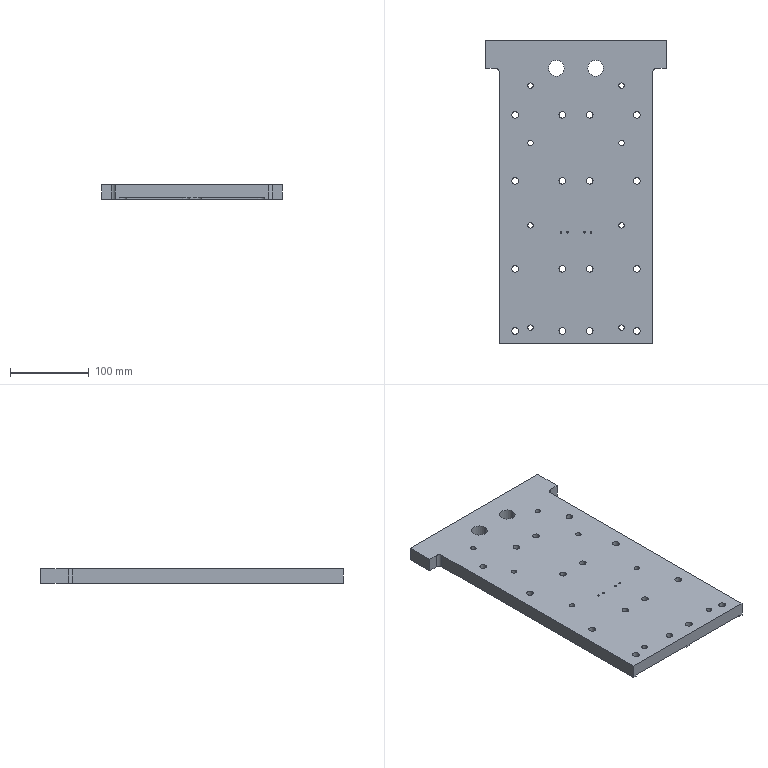NC program | NX | posted with a generic post | part box 230 x 385 x 18 mm
Lines 2114 to 3056 of 3056:
(FLOOR_WALL_COPY , TOOL : D10JING)
N4202 T14 M6
N4204 G54
N4206 G17 G0 G90 X-199. Y86.497 S9500 M3
N4208 G43 Z30. H14
N4210 Z-0.5
N4212 G94 G1 Z-2. F1500.
N4214 X-196.634
N4216 G3 X-197.5 Y86.997 R1.
N4218 G1 X139.033
N4220 G3 X136.7 Y82.5 R5.5
N4222 G1 Y82.06
N4224 X-197.5
N4226 Y77.122
N4228 X136.7
N4230 Y72.185
N4232 X-197.5
N4234 Y67.248
N4236 X136.7
N4238 Y62.31
N4240 X-197.5
N4242 Y57.373
N4244 X136.7
N4246 Y52.436
N4248 X-197.5
N4250 Y47.499
N4252 X136.7
N4254 Y42.561
N4256 X-197.5
N4258 Y37.624
N4260 X136.7
N4262 Y32.687
N4264 X-197.5
N4266 Y27.749
N4268 X136.7
N4270 Y22.812
N4272 X-197.5
N4274 Y17.875
N4276 X136.7
N4278 Y12.937
N4280 X-197.5
N4282 Y8.
N4284 X139.038
N4286 G3 X138.042 Y8.089 R1.
N4288 G1 Z-0.5
N4290 G0 X-199. Y9.098
N4292 G1 Z-2.
N4294 X-198.366 Y8.
N4296 G3 X-197.5 Y7.5 R1.
N4298 G1 X142.2
N4300 G2 X137.2 Y12.5 R5.
N4302 G1 Y82.5
N4304 G2 X142.2 Y87.5 R5.
N4306 G1 X-197.5
N4308 G3 X-198.366 Y87. R1.
N4310 G1 X-199. Y85.902
N4312 Z-0.5
N4314 G0 Z1.1
N4316 Y-8.503
N4318 Z-0.5
N4320 G1 Z-2.
N4322 X-196.634
N4324 G3 X-197.5 Y-8.003 R1.
N4326 G1 X139.033
N4328 G3 X136.7 Y-12.5 R5.5
N4330 G1 Y-12.94
N4332 X-197.5
N4334 Y-17.878
N4336 X136.7
N4338 Y-22.815
N4340 X-197.5
N4342 Y-27.752
N4344 X136.7
N4346 Y-32.69
N4348 X-197.5
N4350 Y-37.627
N4352 X136.7
N4354 Y-42.564
N4356 X-197.5
N4358 Y-47.501
N4360 X136.7
N4362 Y-52.439
N4364 X-197.5
N4366 Y-57.376
N4368 X136.7
N4370 Y-62.313
N4372 X-197.5
N4374 Y-67.251
N4376 X136.7
N4378 Y-72.188
N4380 X-197.5
N4382 Y-77.125
N4384 X136.7
N4386 Y-82.063
N4388 X-197.5
N4390 Y-87.
N4392 X139.038
N4394 G3 X138.042 Y-86.911 R1.
N4396 G1 Z-0.5
N4398 G0 X-199. Y-85.902
N4400 G1 Z-2.
N4402 X-198.366 Y-87.
N4404 G3 X-197.5 Y-87.5 R1.
N4406 G1 X142.2
N4408 G2 X137.2 Y-82.5 R5.
N4410 G1 Y-12.5
N4412 G2 X142.2 Y-7.5 R5.
N4414 G1 X-197.5
N4416 G3 X-198.366 Y-8. R1.
N4418 G1 X-199. Y-9.098
N4420 Z-0.5
N4422 G0 Z30.
(HOLE_MILLING , TOOL : D10JING)
N4424 X157.5 Y25.
N4426 Z0.5
N4428 G3 X160. Y27.5 R2.5 F2200.
N4430 X157.5 Y30. R2.5
N4432 X157.5 Y30. Z-0.38 I0. J-5.
N4434 X157.5 Y30. Z-1.26 I0. J-5.
N4436 X157.5 Y30. Z-2.14 I0. J-5.
N4438 X157.5 Y30. Z-3.02 I0. J-5.
N4440 X157.5 Y30. Z-3.9 I0. J-5.
N4442 X157.5 Y30. Z-4.78 I0. J-5.
N4444 X157.5 Y30. Z-5.66 I0. J-5.
N4446 X157.5 Y30. Z-6.54 I0. J-5.
N4448 X157.5 Y30. Z-7.42 I0. J-5.
N4450 X157.5 Y30. Z-8.3 I0. J-5.
N4452 X157.5 Y30. Z-9.18 I0. J-5.
N4454 X157.5 Y30. Z-10.06 I0. J-5.
N4456 X157.5 Y30. Z-10.94 I0. J-5.
N4458 X157.5 Y30. Z-11.82 I0. J-5.
N4460 X157.5 Y30. Z-12.7 I0. J-5.
N4462 X157.5 Y30. Z-13.58 I0. J-5.
N4464 X157.5 Y30. Z-14.46 I0. J-5.
N4466 X157.5 Y30. Z-15.34 I0. J-5.
N4468 X157.5 Y30. Z-16.22 I0. J-5.
N4470 X157.5 Y30. Z-17.1 I0. J-5.
N4472 X157.5 Y30. Z-17.98 I0. J-5.
N4474 X156.788 Y29.949 Z-18. R5.
N4476 X152.551 Y24.288 R5.
N4478 X156.788 Y29.949 R-5.
N4480 X154.67 Y27.119 R2.5
N4482 X157.5 Y25. R2.5
N4484 G0 Z30.
N4486 Y-25.
N4488 Z0.5
N4490 G3 X160. Y-22.5 R2.5
N4492 X157.5 Y-20. R2.5
N4494 X157.5 Y-20. Z-0.38 I0. J-5.
N4496 X157.5 Y-20. Z-1.26 I0. J-5.
N4498 X157.5 Y-20. Z-2.14 I0. J-5.
N4500 X157.5 Y-20. Z-3.02 I0. J-5.
N4502 X157.5 Y-20. Z-3.9 I0. J-5.
N4504 X157.5 Y-20. Z-4.78 I0. J-5.
N4506 X157.5 Y-20. Z-5.66 I0. J-5.
N4508 X157.5 Y-20. Z-6.54 I0. J-5.
N4510 X157.5 Y-20. Z-7.42 I0. J-5.
N4512 X157.5 Y-20. Z-8.3 I0. J-5.
N4514 X157.5 Y-20. Z-9.18 I0. J-5.
N4516 X157.5 Y-20. Z-10.06 I0. J-5.
N4518 X157.5 Y-20. Z-10.94 I0. J-5.
N4520 X157.5 Y-20. Z-11.82 I0. J-5.
N4522 X157.5 Y-20. Z-12.7 I0. J-5.
N4524 X157.5 Y-20. Z-13.58 I0. J-5.
N4526 X157.5 Y-20. Z-14.46 I0. J-5.
N4528 X157.5 Y-20. Z-15.34 I0. J-5.
N4530 X157.5 Y-20. Z-16.22 I0. J-5.
N4532 X157.5 Y-20. Z-17.1 I0. J-5.
N4534 X157.5 Y-20. Z-17.98 I0. J-5.
N4536 X156.788 Y-20.051 Z-18. R5.
N4538 X152.551 Y-25.712 R5.
N4540 X156.788 Y-20.051 R-5.
N4542 X154.67 Y-22.881 R2.5
N4544 X157.5 Y-25. R2.5
N4546 G0 Z30.
N4548 M5
(PLANAR_MILL_COPY_COPY_COPY , TOOL : D6A45)
N4550 T01 M6
N4552 G54
N4554 G17 G0 G90 X166.1 Y-25.866 S9500 M3
N4556 G43 Z30. H1
N4558 Z0.5
N4560 G94 G1 Z-1. F1250.
N4562 G3 X166.6 Y-25. R1.
N4564 X157.5 Y-15.9 R9.1
N4566 X166.6 Y-25. R-9.1
N4568 X166.1 Y-24.134 R1.
N4570 G1 Z0.5
N4572 G0 Z30.
N4574 Y24.134
N4576 Z0.5
N4578 G1 Z-1.
N4580 G3 X166.6 Y25. R1.
N4582 X157.5 Y34.1 R9.1
N4584 X166.6 Y25. R-9.1
N4586 X166.1 Y25.866 R1.
N4588 G1 Z0.5
N4590 G0 Z30.
N4592 X-20.866 Y98.9
N4594 Z0.5
N4596 G1 Z-1.
N4598 G3 X-20. Y98.4 R1.
N4600 G1 X152.5
N4602 G3 X156.6 Y102.5 R4.1
N4604 G1 Y115.
N4606 G2 X157.5 Y115.9 R0.9
N4608 G1 X192.5
N4610 G2 X193.4 Y115. R0.9
N4612 G1 Y-115.
N4614 G2 X192.5 Y-115.9 R0.9
N4616 G1 X157.5
N4618 G2 X156.6 Y-115. R0.9
N4620 G1 Y-102.5
N4622 G3 X152.5 Y-98.4 R4.1
N4624 G1 X-192.5
N4626 G2 X-193.4 Y-97.5 R0.9
N4628 G1 Y-92.5
N4630 G2 X-192.5 Y-91.6 R0.9
N4632 G1 X142.2
N4634 G3 X146.3 Y-87.5 R4.1
N4636 X142.2 Y-83.4 R4.1
N4638 G2 X141.3 Y-82.5 R0.9
N4640 G1 Y-12.5
N4642 G2 X142.2 Y-11.6 R0.9
N4644 G3 X146.3 Y-7.5 R4.1
N4646 X142.2 Y-3.4 R4.1
N4648 G1 X-192.5
N4650 G2 X-193.4 Y-2.5 R0.9
N4652 G1 Y2.5
N4654 G2 X-192.5 Y3.4 R0.9
N4656 G1 X142.2
N4658 G3 X146.3 Y7.5 R4.1
N4660 X142.2 Y11.6 R4.1
N4662 G2 X141.3 Y12.5 R0.9
N4664 G1 Y82.5
N4666 G2 X142.2 Y83.4 R0.9
N4668 G3 X146.3 Y87.5 R4.1
N4670 X142.2 Y91.6 R4.1
N4672 G1 X-192.5
N4674 G2 X-193.4 Y92.5 R0.9
N4676 G1 Y97.5
N4678 G2 X-192.5 Y98.4 R0.9
N4680 G1 X-20.
N4682 G3 X-19.134 Y98.9 R1.
N4684 G1 Z0.5
N4686 G0 Z30.
N4688 M5
(FLOOR_WALL_COPY_COPY , TOOL : D10JING)
N4690 T14 M6
N4692 G54
N4694 G17 G0 G90 X-198.978 Y9.094 S9500 M3
N4696 G43 Z30. H14
N4698 Z-0.5
N4700 G94 G1 Z-2. F1500.
N4702 G41 X-198.943 Y9. D14
N4704 X-198.366 Y8.
N4706 G3 X-197.5 Y7.5 R1.
N4708 G1 X142.2
N4710 G2 X137.2 Y12.5 R5.
N4712 G1 Y82.5
N4714 G2 X142.2 Y87.5 R5.
N4716 G1 X-197.5
N4718 G3 X-198.366 Y87. R1.
N4720 G1 X-198.943 Y86.
N4722 G40
N4724 X-198.978 Y85.906
N4726 Z-0.5
N4728 G0 Z1.1
N4730 Y-85.906
N4732 Z-0.5
N4734 G1 Z-2.
N4736 G41 X-198.943 Y-86.
N4738 X-198.366 Y-87.
N4740 G3 X-197.5 Y-87.5 R1.
N4742 G1 X142.2
N4744 G2 X137.2 Y-82.5 R5.
N4746 G1 Y-12.5
N4748 G2 X142.2 Y-7.5 R5.
N4750 G1 X-197.5
N4752 G3 X-198.366 Y-8. R1.
N4754 G1 X-198.943 Y-9.
N4756 G40
N4758 X-198.978 Y-9.094
N4760 Z-0.5
N4762 G0 Z30.
N4764 M5
(PLANAR_MILL_COPY_COPY_COPY_COPY , TOOL : D6A45)
N4766 T01 M6
N4768 G54
N4770 G17 G0 G90 X-178.857 Y-76.875 S9500 M3
N4772 G43 Z30. H1
N4774 Z-1.5
N4776 G94 G1 Z-3. F1250.
N4778 X-179.65 Y-76.634
N4780 G3 X-180.15 Y-77.5 R1.
N4782 X-176.8 Y-80.85 R3.35
N4784 X-180.15 Y-77.5 R-3.35
N4786 X-179.65 Y-78.366 R1.
N4788 G1 X-178.857 Y-78.125
N4790 Z-1.5
N4792 G0 Z30.
N4794 X-173.693 Y-57.483
N4796 Z-1.5
N4798 G1 Z-3.
N4800 X-174.5 Y-57.134
N4802 G3 X-175. Y-58. R1.
N4804 X-172.5 Y-60.5 R2.5
N4806 X-175. Y-58. R-2.5
N4808 X-174.5 Y-58.866 R1.
N4810 G1 X-173.693 Y-58.517
N4812 Z-1.5
N4814 G0 Z30.
N4816 X-178.857 Y-16.875
N4818 Z-1.5
N4820 G1 Z-3.
N4822 X-179.65 Y-16.634
N4824 G3 X-180.15 Y-17.5 R1.
N4826 X-176.8 Y-20.85 R3.35
N4828 X-180.15 Y-17.5 R-3.35
N4830 X-179.65 Y-18.366 R1.
N4832 G1 X-178.857 Y-18.125
N4834 Z-1.5
N4836 G0 Z30.
N4838 Y18.125
N4840 Z-1.5
N4842 G1 Z-3.
N4844 X-179.65 Y18.366
N4846 G3 X-180.15 Y17.5 R1.
N4848 X-176.8 Y14.15 R3.35
N4850 X-180.15 Y17.5 R-3.35
N4852 X-179.65 Y16.634 R1.
N4854 G1 X-178.857 Y16.875
N4856 Z-1.5
N4858 G0 Z30.
N4860 X-173.693 Y58.517
N4862 Z-1.5
N4864 G1 Z-3.
N4866 X-174.5 Y58.866
N4868 G3 X-175. Y58. R1.
N4870 X-172.5 Y55.5 R2.5
N4872 X-175. Y58. R-2.5
N4874 X-174.5 Y57.134 R1.
N4876 G1 X-173.693 Y57.483
N4878 Z-1.5
N4880 G0 Z30.
N4882 X-178.857 Y78.125
N4884 Z-1.5
N4886 G1 Z-3.
N4888 X-179.65 Y78.366
N4890 G3 X-180.15 Y77.5 R1.
N4892 X-176.8 Y74.15 R3.35
N4894 X-180.15 Y77.5 R-3.35
N4896 X-179.65 Y76.634 R1.
N4898 G1 X-178.857 Y76.875
N4900 Z-1.5
N4902 G0 Z30.
N4904 X-97.175 Y79.557
N4906 Z-1.5
N4908 G1 Z-3.
N4910 X-96.934 Y80.35
N4912 G3 X-97.8 Y80.85 R1.
N4914 X-101.15 Y77.5 R3.35
N4916 X-97.8 Y80.85 R-3.35
N4918 X-98.666 Y80.35 R1.
N4920 G1 X-98.425 Y79.557
N4922 Z-1.5
N4924 G0 Z30.
N4926 X-41.983 Y59.193
N4928 Z-1.5
N4930 G1 Z-3.
N4932 X-41.634 Y60.
N4934 G3 X-42.5 Y60.5 R1.
N4936 X-45. Y58. R2.5
N4938 X-42.5 Y60.5 R-2.5
N4940 X-43.366 Y60. R1.
N4942 G1 X-43.017 Y59.193
N4944 Z-1.5
N4946 G0 Z30.
N4948 X-99.857 Y18.125
N4950 Z-1.5
N4952 G1 Z-3.
N4954 X-100.65 Y18.366
N4956 G3 X-101.15 Y17.5 R1.
N4958 X-97.8 Y14.15 R3.35
N4960 X-101.15 Y17.5 R-3.35
N4962 X-100.65 Y16.634 R1.
N4964 G1 X-99.857 Y16.875
N4966 Z-1.5
N4968 G0 Z30.
N4970 Y-16.875
N4972 Z-1.5
N4974 G1 Z-3.
N4976 X-100.65 Y-16.634
N4978 G3 X-101.15 Y-17.5 R1.
N4980 X-97.8 Y-20.85 R3.35
N4982 X-101.15 Y-17.5 R-3.35
N4984 X-100.65 Y-18.366 R1.
N4986 G1 X-99.857 Y-18.125
N4988 Z-1.5
N4990 G0 Z30.
N4992 X-98.425 Y-79.557
N4994 Z-1.5
N4996 G1 Z-3.
N4998 X-98.666 Y-80.35
N5000 G3 X-97.8 Y-80.85 R1.
N5002 X-94.45 Y-77.5 R3.35
N5004 X-97.8 Y-80.85 R-3.35
N5006 X-96.934 Y-80.35 R1.
N5008 G1 X-97.175 Y-79.557
N5010 Z-1.5
N5012 G0 Z30.
N5014 X-43.017 Y-59.193
N5016 Z-1.5
N5018 G1 Z-3.
N5020 X-43.366 Y-60.
N5022 G3 X-42.5 Y-60.5 R1.
N5024 X-40. Y-58. R2.5
N5026 X-42.5 Y-60.5 R-2.5
N5028 X-41.634 Y-60. R1.
N5030 G1 X-41.983 Y-59.193
N5032 Z-1.5
N5034 G0 Z30.
N5036 X13.575 Y-79.557
N5038 Z-1.5
N5040 G1 Z-3.
N5042 X13.334 Y-80.35
N5044 G3 X14.2 Y-80.85 R1.
N5046 X17.55 Y-77.5 R3.35
N5048 X14.2 Y-80.85 R-3.35
N5050 X15.066 Y-80.35 R1.
N5052 G1 X14.825 Y-79.557
N5054 Z-1.5
N5056 G0 Z30.
N5058 X61.983 Y-59.193
N5060 Z-1.5
N5062 G1 Z-3.
N5064 X61.634 Y-60.
N5066 G3 X62.5 Y-60.5 R1.
N5068 X65. Y-58. R2.5
N5070 X62.5 Y-60.5 R-2.5
N5072 X63.366 Y-60. R1.
N5074 G1 X63.017 Y-59.193
N5076 Z-1.5
N5078 G0 Z30.
N5080 X97.575 Y-79.557
N5082 Z-1.5
N5084 G1 Z-3.
N5086 X97.334 Y-80.35
N5088 G3 X98.2 Y-80.85 R1.
N5090 X101.55 Y-77.5 R3.35
N5092 X98.2 Y-80.85 R-3.35
N5094 X99.066 Y-80.35 R1.
N5096 G1 X98.825 Y-79.557
N5098 Z-1.5
N5100 G0 Z30.
N5102 X134.983 Y-59.193
N5104 Z-1.5
N5106 G1 Z-3.
N5108 X134.634 Y-60.
N5110 G3 X135.5 Y-60.5 R1.
N5112 X138. Y-58. R2.5
N5114 X135.5 Y-60.5 R-2.5
N5116 X136.366 Y-60. R1.
N5118 G1 X136.017 Y-59.193
N5120 Z-1.5
N5122 G0 Z30.
N5124 X100.257 Y-18.125
N5126 Z-1.5
N5128 G1 Z-3.
N5130 X101.05 Y-18.366
N5132 G3 X101.55 Y-17.5 R1.
N5134 X98.2 Y-14.15 R3.35
N5136 X101.55 Y-17.5 R-3.35
N5138 X101.05 Y-16.634 R1.
N5140 G1 X100.257 Y-16.875
N5142 Z-1.5
N5144 G0 Z30.
N5146 Y16.875
N5148 Z-1.5
N5150 G1 Z-3.
N5152 X101.05 Y16.634
N5154 G3 X101.55 Y17.5 R1.
N5156 X98.2 Y20.85 R3.35
N5158 X101.55 Y17.5 R-3.35
N5160 X101.05 Y18.366 R1.
N5162 G1 X100.257 Y18.125
N5164 Z-1.5
N5166 G0 Z30.
N5168 X136.017 Y59.193
N5170 Z-1.5
N5172 G1 Z-3.
N5174 X136.366 Y60.
N5176 G3 X135.5 Y60.5 R1.
N5178 X133. Y58. R2.5
N5180 X135.5 Y60.5 R-2.5
N5182 X134.634 Y60. R1.
N5184 G1 X134.983 Y59.193
N5186 Z-1.5
N5188 G0 Z30.
N5190 X98.825 Y79.557
N5192 Z-1.5
N5194 G1 Z-3.
N5196 X99.066 Y80.35
N5198 G3 X98.2 Y80.85 R1.
N5200 X94.85 Y77.5 R3.35
N5202 X98.2 Y80.85 R-3.35
N5204 X97.334 Y80.35 R1.
N5206 G1 X97.575 Y79.557
N5208 Z-1.5
N5210 G0 Z30.
N5212 X63.017 Y59.193
N5214 Z-1.5
N5216 G1 Z-3.
N5218 X63.366 Y60.
N5220 G3 X62.5 Y60.5 R1.
N5222 X60. Y58. R2.5
N5224 X62.5 Y60.5 R-2.5
N5226 X61.634 Y60. R1.
N5228 G1 X61.983 Y59.193
N5230 Z-1.5
N5232 G0 Z30.
N5234 X14.825 Y79.557
N5236 Z-1.5
N5238 G1 Z-3.
N5240 X15.066 Y80.35
N5242 G3 X14.2 Y80.85 R1.
N5244 X10.85 Y77.5 R3.35
N5246 X14.2 Y80.85 R-3.35
N5248 X13.334 Y80.35 R1.
N5250 G1 X13.575 Y79.557
N5252 Z-1.5
N5254 G0 Z30.
N5256 X14.825 Y19.557
N5258 Z-1.5
N5260 G1 Z-3.
N5262 X15.066 Y20.35
N5264 G3 X14.2 Y20.85 R1.
N5266 X10.85 Y17.5 R3.35
N5268 X14.2 Y20.85 R-3.35
N5270 X13.334 Y20.35 R1.
N5272 G1 X13.575 Y19.557
N5274 Z-1.5
N5276 G0 Z30.
N5278 X-194.813 Y6.592
N5280 Z-1.5
N5282 G1 Z-3.
N5284 X-194.365 Y6.143
N5286 G3 X-193.4 Y5.882 R1.
N5288 G1 Y89.118
N5290 G3 X-194.365 Y88.857 R1.
N5292 G1 X-194.813 Y88.408
N5294 Z-1.5
N5296 G0 Z30.
N5298 Y-88.408
N5300 Z-1.5
N5302 G1 Z-3.
N5304 X-194.365 Y-88.857
N5306 G3 X-193.4 Y-89.118 R1.
N5308 G1 Y-5.882
N5310 G3 X-194.365 Y-6.143 R1.
N5312 G1 X-194.813 Y-6.592
N5314 Z-1.5
N5316 G0 Z30.
N5318 X13.575 Y-19.557
N5320 Z-1.5
N5322 G1 Z-3.
N5324 X13.334 Y-20.35
N5326 G3 X14.2 Y-20.85 R1.
N5328 X17.55 Y-17.5 R3.35
N5330 X14.2 Y-20.85 R-3.35
N5332 X15.066 Y-20.35 R1.
N5334 G1 X14.825 Y-19.557
N5336 Z-1.5
N5338 G0 Z30.
N5340 M5
(ZLEVEL_PROFILE_COPY_1 , TOOL : D10JING)
N5342 T14 M6
N5344 G54
N5346 G17 G0 G90 X-51.007 Y102.5 S9500 M3
N5348 G43 Z30. H14
N5350 Z-15.9
N5352 G94 G1 X-20. Z-17.525 F1000.
N5354 X152.5 F1200.
N5356 Y115.
N5358 G2 X157.5 Y120. R5.
N5360 G1 X192.5
N5362 G2 X197.5 Y115. R5.
N5364 G1 Y-115.
N5366 G2 X192.5 Y-120. R5.
N5368 G1 X157.5
N5370 G2 X152.5 Y-115. R5.
N5372 G1 Y-102.5
N5374 X-192.5
N5376 G2 X-197.5 Y-97.5 R5.
N5378 G1 Y97.5
N5380 G2 X-192.5 Y102.5 R5.
N5382 G1 X-20.
N5384 X152.5 Z-17.542
N5386 Y115. Z-17.543
N5388 X152.524 Y115.49
N5390 X152.596 Y115.975
N5392 X152.715 Y116.451 Z-17.544
N5394 X152.881 Y116.913
N5396 X153.09 Y117.357
N5398 X153.343 Y117.778
N5400 X153.635 Y118.172
N5402 X153.964 Y118.536
N5404 X154.328 Y118.865
N5406 X154.722 Y119.157
N5408 X155.143 Y119.41
N5410 X155.587 Y119.619
N5412 X156.049 Y119.785
N5414 X156.525 Y119.904
N5416 X157.01 Y119.976
N5418 X157.5 Y120.
N5420 X192.5 Z-17.548
N5422 X192.99 Y119.976
N5424 X193.475 Y119.904
N5426 X193.951 Y119.785
N5428 X194.413 Y119.619
N5430 X194.857 Y119.41
N5432 X195.278 Y119.157
N5434 X195.672 Y118.865
N5436 X196.036 Y118.536
N5438 X196.365 Y118.172
N5440 X196.657 Y117.778
N5442 X196.91 Y117.357
N5444 X197.119 Y116.913
N5446 X197.285 Y116.451
N5448 X197.404 Y115.975
N5450 X197.476 Y115.49
N5452 X197.5 Y115.
N5454 Y-115. Z-17.571
N5456 X197.476 Y-115.49
N5458 X197.404 Y-115.975
N5460 X197.285 Y-116.451
N5462 X197.119 Y-116.913 Z-17.572
N5464 X196.91 Y-117.357
N5466 X196.657 Y-117.778
N5468 X196.365 Y-118.172
N5470 X196.036 Y-118.536
N5472 X195.672 Y-118.865
N5474 X195.278 Y-119.157
N5476 X194.857 Y-119.41
N5478 X194.413 Y-119.619
N5480 X193.951 Y-119.785
N5482 X193.475 Y-119.904
N5484 X192.99 Y-119.976
N5486 X192.5 Y-120.
N5488 X157.5 Z-17.576
N5490 X157.01 Y-119.976
N5492 X156.525 Y-119.904
N5494 X156.049 Y-119.785
N5496 X155.587 Y-119.619
N5498 X155.143 Y-119.41
N5500 X154.722 Y-119.157
N5502 X154.328 Y-118.865
N5504 X153.964 Y-118.536
N5506 X153.635 Y-118.172
N5508 X153.343 Y-117.778
N5510 X153.09 Y-117.357
N5512 X152.881 Y-116.913
N5514 X152.715 Y-116.451
N5516 X152.596 Y-115.975
N5518 X152.524 Y-115.49
N5520 X152.5 Y-115.
N5522 Y-102.5 Z-17.578
N5524 X-192.5 Z-17.612
N5526 X-192.99 Y-102.476
N5528 X-193.475 Y-102.404
N5530 X-193.951 Y-102.285
N5532 X-194.413 Y-102.119
N5534 X-194.857 Y-101.91
N5536 X-195.278 Y-101.657
N5538 X-195.672 Y-101.365
N5540 X-196.036 Y-101.036
N5542 X-196.365 Y-100.672
N5544 X-196.657 Y-100.278
N5546 X-196.91 Y-99.857
N5548 X-197.119 Y-99.413
N5550 X-197.285 Y-98.951 Z-17.613
N5552 X-197.404 Y-98.475
N5554 X-197.476 Y-97.99
N5556 X-197.5 Y-97.5
N5558 Y97.5 Z-17.632
N5560 X-197.476 Y97.99
N5562 X-197.404 Y98.475
N5564 X-197.285 Y98.951
N5566 X-197.119 Y99.413
N5568 X-196.91 Y99.857
N5570 X-196.657 Y100.278
N5572 X-196.365 Y100.672
N5574 X-196.036 Y101.036
N5576 X-195.672 Y101.365 Z-17.633
N5578 X-195.278 Y101.657
N5580 X-194.857 Y101.91
N5582 X-194.413 Y102.119
N5584 X-193.951 Y102.285
N5586 X-193.475 Y102.404
N5588 X-192.99 Y102.476
N5590 X-192.5 Y102.5
N5592 X-20. Z-17.65
N5594 X152.5 Z-17.667
N5596 Y115. Z-17.668
N5598 X152.524 Y115.49
N5600 X152.596 Y115.975
N5602 X152.715 Y116.451 Z-17.669
N5604 X152.881 Y116.913
N5606 X153.09 Y117.357
N5608 X153.343 Y117.778
N5610 X153.635 Y118.172
N5612 X153.964 Y118.536
N5614 X154.328 Y118.865
N5616 X154.722 Y119.157
N5618 X155.143 Y119.41
N5620 X155.587 Y119.619
N5622 X156.049 Y119.785
N5624 X156.525 Y119.904
N5626 X157.01 Y119.976
N5628 X157.5 Y120.
N5630 X192.5 Z-17.673
N5632 X192.99 Y119.976
N5634 X193.475 Y119.904
N5636 X193.951 Y119.785
N5638 X194.413 Y119.619
N5640 X194.857 Y119.41
N5642 X195.278 Y119.157
N5644 X195.672 Y118.865
N5646 X196.036 Y118.536
N5648 X196.365 Y118.172
N5650 X196.657 Y117.778
N5652 X196.91 Y117.357
N5654 X197.119 Y116.913
N5656 X197.285 Y116.451
N5658 X197.404 Y115.975
N5660 X197.476 Y115.49
N5662 X197.5 Y115.
N5664 Y-115. Z-17.696
N5666 X197.476 Y-115.49
N5668 X197.404 Y-115.975
N5670 X197.285 Y-116.451
N5672 X197.119 Y-116.913 Z-17.697
N5674 X196.91 Y-117.357
N5676 X196.657 Y-117.778
N5678 X196.365 Y-118.172
N5680 X196.036 Y-118.536
N5682 X195.672 Y-118.865
N5684 X195.278 Y-119.157
N5686 X194.857 Y-119.41
N5688 X194.413 Y-119.619
N5690 X193.951 Y-119.785
N5692 X193.475 Y-119.904
N5694 X192.99 Y-119.976
N5696 X192.5 Y-120.
N5698 X157.5 Z-17.701
N5700 X157.01 Y-119.976
N5702 X156.525 Y-119.904
N5704 X156.049 Y-119.785
N5706 X155.587 Y-119.619
N5708 X155.143 Y-119.41
N5710 X154.722 Y-119.157
N5712 X154.328 Y-118.865
N5714 X153.964 Y-118.536
N5716 X153.635 Y-118.172
N5718 X153.343 Y-117.778
N5720 X153.09 Y-117.357
N5722 X152.881 Y-116.913
N5724 X152.715 Y-116.451
N5726 X152.596 Y-115.975
N5728 X152.524 Y-115.49
N5730 X152.5 Y-115.
N5732 Y-102.5 Z-17.703
N5734 X-192.5 Z-17.737
N5736 X-192.99 Y-102.476
N5738 X-193.475 Y-102.404
N5740 X-193.951 Y-102.285
N5742 X-194.413 Y-102.119
N5744 X-194.857 Y-101.91
N5746 X-195.278 Y-101.657
N5748 X-195.672 Y-101.365
N5750 X-196.036 Y-101.036
N5752 X-196.365 Y-100.672
N5754 X-196.657 Y-100.278
N5756 X-196.91 Y-99.857
N5758 X-197.119 Y-99.413
N5760 X-197.285 Y-98.951 Z-17.738
N5762 X-197.404 Y-98.475
N5764 X-197.476 Y-97.99
N5766 X-197.5 Y-97.5
N5768 Y97.5 Z-17.757
N5770 X-197.476 Y97.99
N5772 X-197.404 Y98.475
N5774 X-197.285 Y98.951
N5776 X-197.119 Y99.413
N5778 X-196.91 Y99.857
N5780 X-196.657 Y100.278
N5782 X-196.365 Y100.672
N5784 X-196.036 Y101.036
N5786 X-195.672 Y101.365 Z-17.758
N5788 X-195.278 Y101.657
N5790 X-194.857 Y101.91
N5792 X-194.413 Y102.119
N5794 X-193.951 Y102.285
N5796 X-193.475 Y102.404
N5798 X-192.99 Y102.476
N5800 X-192.5 Y102.5
N5802 X-20. Z-17.775
N5804 X152.5 Z-17.792
N5806 Y115. Z-17.793
N5808 X152.524 Y115.49
N5810 X152.596 Y115.975
N5812 X152.715 Y116.451 Z-17.794
N5814 X152.881 Y116.913
N5816 X153.09 Y117.357
N5818 X153.343 Y117.778
N5820 X153.635 Y118.172
N5822 X153.964 Y118.536
N5824 X154.328 Y118.865
N5826 X154.722 Y119.157
N5828 X155.143 Y119.41
N5830 X155.587 Y119.619
N5832 X156.049 Y119.785
N5834 X156.525 Y119.904
N5836 X157.01 Y119.976
N5838 X157.5 Y120.
N5840 X192.5 Z-17.798
N5842 X192.99 Y119.976
N5844 X193.475 Y119.904
N5846 X193.951 Y119.785
N5848 X194.413 Y119.619
N5850 X194.857 Y119.41
N5852 X195.278 Y119.157
N5854 X195.672 Y118.865
N5856 X196.036 Y118.536
N5858 X196.365 Y118.172
N5860 X196.657 Y117.778
N5862 X196.91 Y117.357
N5864 X197.119 Y116.913
N5866 X197.285 Y116.451
N5868 X197.404 Y115.975
N5870 X197.476 Y115.49
N5872 X197.5 Y115.
N5874 Y-115. Z-17.821
N5876 X197.476 Y-115.49
N5878 X197.404 Y-115.975
N5880 X197.285 Y-116.451
N5882 X197.119 Y-116.913 Z-17.822
N5884 X196.91 Y-117.357
N5886 X196.657 Y-117.778
N5888 X196.365 Y-118.172
N5890 X196.036 Y-118.536
N5892 X195.672 Y-118.865
N5894 X195.278 Y-119.157
N5896 X194.857 Y-119.41
N5898 X194.413 Y-119.619
N5900 X193.951 Y-119.785
N5902 X193.475 Y-119.904
N5904 X192.99 Y-119.976
N5906 X192.5 Y-120.
N5908 X157.5 Z-17.826
N5910 X157.01 Y-119.976
N5912 X156.525 Y-119.904
N5914 X156.049 Y-119.785
N5916 X155.587 Y-119.619
N5918 X155.143 Y-119.41
N5920 X154.722 Y-119.157
N5922 X154.328 Y-118.865
N5924 X153.964 Y-118.536
N5926 X153.635 Y-118.172
N5928 X153.343 Y-117.778
N5930 X153.09 Y-117.357
N5932 X152.881 Y-116.913
N5934 X152.715 Y-116.451
N5936 X152.596 Y-115.975
N5938 X152.524 Y-115.49
N5940 X152.5 Y-115.
N5942 Y-102.5 Z-17.828
N5944 X-192.5 Z-17.862
N5946 X-192.99 Y-102.476
N5948 X-193.475 Y-102.404
N5950 X-193.951 Y-102.285
N5952 X-194.413 Y-102.119
N5954 X-194.857 Y-101.91
N5956 X-195.278 Y-101.657
N5958 X-195.672 Y-101.365
N5960 X-196.036 Y-101.036
N5962 X-196.365 Y-100.672
N5964 X-196.657 Y-100.278
N5966 X-196.91 Y-99.857
N5968 X-197.119 Y-99.413
N5970 X-197.285 Y-98.951 Z-17.863
N5972 X-197.404 Y-98.475
N5974 X-197.476 Y-97.99
N5976 X-197.5 Y-97.5
N5978 Y97.5 Z-17.882
N5980 X-197.476 Y97.99
N5982 X-197.404 Y98.475
N5984 X-197.285 Y98.951
N5986 X-197.119 Y99.413
N5988 X-196.91 Y99.857
N5990 X-196.657 Y100.278
N5992 X-196.365 Y100.672
N5994 X-196.036 Y101.036
N5996 X-195.672 Y101.365 Z-17.883
N5998 X-195.278 Y101.657
N6000 X-194.857 Y101.91
N6002 X-194.413 Y102.119
N6004 X-193.951 Y102.285
N6006 X-193.475 Y102.404
N6008 X-192.99 Y102.476
N6010 X-192.5 Y102.5
N6012 X-20. Z-17.9
N6014 X152.5
N6016 Y115.
N6018 G2 X157.5 Y120. R5.
N6020 G1 X192.5
N6022 G2 X197.5 Y115. R5.
N6024 G1 Y-115.
N6026 G2 X192.5 Y-120. R5.
N6028 G1 X157.5
N6030 G2 X152.5 Y-115. R5.
N6032 G1 Y-102.5
N6034 X-192.5
N6036 G2 X-197.5 Y-97.5 R5.
N6038 G1 Y97.5
N6040 G2 X-192.5 Y102.5 R5.
N6042 G1 X-20.
N6044 Z-16.4
N6046 G0 Z30.
N6048 M5
N6050 M2